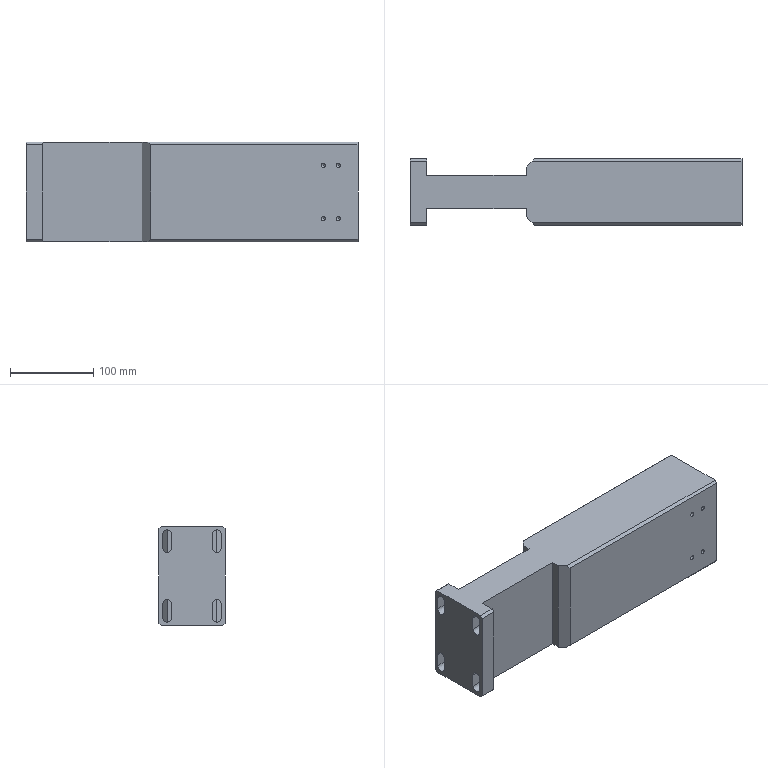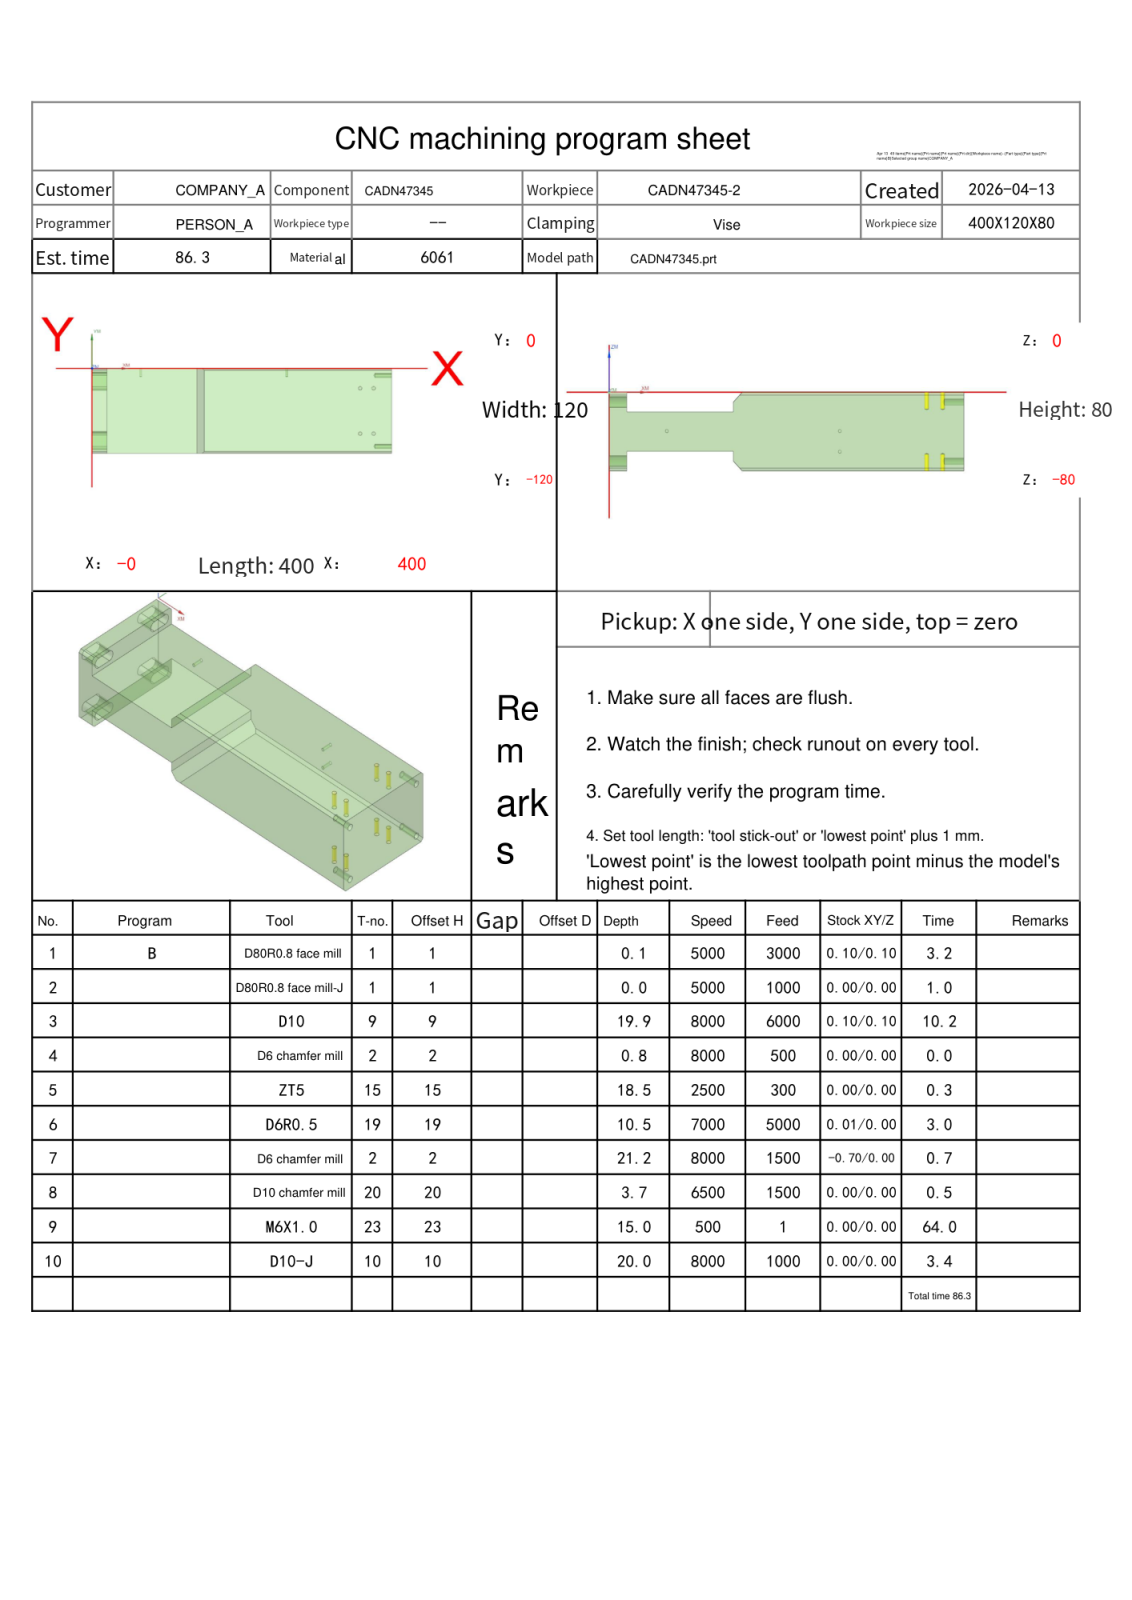NC program | NX | posted by the shop | part box 400 x 80 x 120 mm
Lines 148 to 1360 of 4568:
N3 T09 M06
(D10  D=10. R=0. H=09 ce=0.10 di=0.10)
G00 G90 G54 X91.621 Y-134.5 M03 S8000
G43 H09 Z14.8
M08
Z.404
G01 Z-.796 F6000.
Y-127.08
G03 X84.621 Y-120.08 I-7. J0.0
G01 X26.087
X25.177
G02 X24.48 Y-122.521 I-5.247 J.18
X24.167 Y-123. I-4.55 J2.62
G01 X23.918
G02 X20. Y-124.337 I-3.965 J5.21
G01 X.08
Y-123.
X-.08
Y-122.937
X.08 Y-122.938
X1.48 Y-122.937
X20.
G03 X25.099 Y-117.903 I-.047 J5.147
G01 X25.117 Y-117.802
X25.179 Y-117.08
X25.18 Y-116.774
Y-116.579
Y-116.189
Y-114.405
X25.179 Y-113.513
Y-3.812
X25.178 Y-2.913
X25.116 Y-2.19
X25.099 Y-2.097
G03 X20. Y2.937 I-5.146 J-.113
G01 X1.48
X.08 Y2.938
X-.08 Y2.937
Y3.
X.08
Y4.337
X20.013
G02 X23.918 Y3. I-.06 J-6.547
G01 X24.154
G02 X24.452 Y2.547 I-4.274 J-3.135
X25.176 Y.08 I-4.572 J-2.682
G01 X26.087
X134.898
X135.207
X141.852
G02 X142.877 Y3. I5.492 J-.286
G01 X145.194
G02 X149.133 Y4.337 I3.939 J-5.134
G01 X399.92
Y3.
X400.08
Y2.937
X399.92 Y2.938
X149.133 Y2.937
G03 X144.063 Y-2.133 I0.0 J-5.071
G01 Y-117.867
G03 X149.133 Y-122.937 I5.071 J0.0
G01 X398.52
X399.92
X400.08
Y-123.
X399.92
Y-124.337
X149.133
G02 X145.194 Y-123. I0.0 J6.471
G01 X142.86
G02 X142.513 Y-122.469 I4.246 J3.15
G01 X142.281 Y-122.023
X142.117 Y-121.559
X141.891 Y-120.662
X141.789 Y-120.08
X135.207
X134.898
X87.635
G02 X86.822 Y-119.662 I.001 J1.
G01 X82.419 Y-113.498
G03 X81.607 Y-113.08 I-.813 J-.582
G01 X33.175
G02 X32.179 Y-112.084 I.004 J1.
G01 Y-7.916
G02 X33.175 Y-6.92 I1. J-.004
G01 X134.896
X135.205
X136.067
G02 X137.063 Y-7.916 I-.004 J-1.
G01 Y-112.084
G02 X136.067 Y-113.08 I-1. J.004
G01 X135.205
X134.896
X87.635
G02 X86.822 Y-112.662 I.001 J1.
G01 X82.419 Y-106.498
G03 X81.606 Y-106.08 I-.813 J-.582
G01 X40.174
G02 X39.179 Y-105.085 I.005 J1.
G01 Y-14.915
G02 X40.174 Y-13.92 I1. J-.005
G01 X129.067
G02 X130.063 Y-14.915 I-.005 J-1.
G01 Y-105.085
G02 X129.067 Y-106.08 I-1. J.005
G01 X87.635
G02 X86.822 Y-105.662 I.001 J1.
G01 X82.419 Y-99.498
G03 X81.606 Y-99.08 I-.813 J-.582
G01 X47.174
G02 X46.179 Y-98.085 I.005 J1.
G01 Y-21.915
G02 X47.174 Y-20.92 I1. J-.005
G01 X122.067
G02 X123.063 Y-21.915 I-.005 J-1.
G01 Y-98.085
G02 X122.067 Y-99.08 I-1. J.005
G01 X87.635
G02 X86.822 Y-98.662 I0.0 J1.
G01 X82.419 Y-92.498
G03 X81.606 Y-92.08 I-.813 J-.582
G01 X54.174
G02 X53.179 Y-91.085 I.005 J1.
G01 Y-28.915
G02 X54.174 Y-27.92 I1. J-.005
G01 X115.068
G02 X116.063 Y-28.915 I-.005 J-1.
G01 Y-91.085
G02 X115.068 Y-92.08 I-1. J.005
G01 X87.635
G02 X86.822 Y-91.662 I0.0 J1.
G01 X82.419 Y-85.498
G03 X81.606 Y-85.08 I-.814 J-.582
G01 X61.173
G02 X60.179 Y-84.085 I.005 J1.
G01 Y-35.915
G02 X61.173 Y-34.92 I1. J-.005
G01 X108.068
G02 X109.063 Y-35.915 I-.005 J-1.
G01 Y-84.085
G02 X108.068 Y-85.08 I-1. J.005
G01 X87.635
G02 X86.822 Y-84.662 I0.0 J1.
G01 X82.419 Y-78.498
G03 X81.606 Y-78.08 I-.814 J-.582
G01 X68.173
G02 X67.179 Y-77.085 I.005 J1.
G01 Y-42.915
G02 X68.173 Y-41.92 I1. J-.005
G01 X101.068
G02 X102.063 Y-42.915 I-.005 J-1.
G01 Y-77.085
G02 X101.068 Y-78.08 I-1. J.005
G01 X87.635
G02 X86.822 Y-77.662 I0.0 J1.
G01 X82.42 Y-71.499
G03 X81.606 Y-71.08 I-.814 J-.582
G01 X75.173
G02 X74.179 Y-70.085 I.005 J1.
G01 Y-49.915
G02 X75.173 Y-48.92 I1. J-.005
G01 X94.068
G02 X95.063 Y-49.915 I-.005 J-1.
G01 Y-70.085
G02 X94.068 Y-71.08 I-1. J.005
G01 X87.635
G02 X86.822 Y-70.661 I0.0 J1.
G01 X82.344 Y-64.391
G03 X81.854 Y-64.026 I-.814 J-.581
G02 X81.179 Y-63.085 I.324 J.946
G01 Y-56.915
G02 X82.173 Y-55.92 I1. J-.005
G01 X87.068
G02 X88.063 Y-56.915 I-.005 J-1.
G01 Y-63.085
G02 X87.068 Y-64.08 I-1. J.005
G01 X84.621
X84.121
G03 X77.121 Y-71.08 I0.0 J-7.
G01 Z.404
G00 Z3.
G01 X91.621 Y-134.5
G00 Z-.392
G01 Z-1.592
Y-127.08
G03 X84.621 Y-120.08 I-7. J0.0
G01 X25.177
G02 X19.93 Y-125.151 I-5.247 J.18
G01 X19.92
X0.0
X-.085 Y-125.156
X-.08 Y-125.071
Y-123.733
X0.0
X.003
X.08
X20.
G03 X25.1 Y-118.613 I-.021 J5.121
G01 Y-118.592
Y-117.897
X25.117 Y-117.802
X25.179 Y-117.08
X25.18 Y-116.774
Y-116.579
Y-116.189
Y-115.297
Y-114.405
X25.179 Y-113.513
Y-3.812
X25.178 Y-2.913
X25.116 Y-2.19
X25.1 Y-2.103
Y-1.408
Y-1.387
G03 X20. Y3.733 I-5.121 J0.0
G01 X.08
X.007
X0.0
X-.08
Y5.071
X-.085 Y5.156
X0.0 Y5.151
X19.922
X20.504 Y5.134
X20.828 Y5.08
G02 X25.176 Y.08 I-.948 J-5.215
G01 X33.175
X134.898
X135.27
X141.852
G02 X144.103 Y4.236 I5.492 J-.287
X147.426 Y5.157 I3.324 J-5.531
X147.72 Y5.151 I0.0 J-6.453
G01 X400.
X400.085 Y5.156
X400.08 Y5.071
Y3.733
X400.
X399.994
X399.92
X148.337
G03 X143.267 Y-1.337 I0.0 J-5.071
G01 Y-118.663
G03 X148.337 Y-123.733 I5.071 J0.0
G01 X399.92
X400.08
Y-124.215
Y-125.071
X400.085 Y-125.156
X400. Y-125.151
X147.717
X146.821 Y-125.129
G02 X142.513 Y-122.469 I.285 J5.279
G01 X142.281 Y-122.023
X142.117 Y-121.559
X141.891 Y-120.662
X141.789 Y-120.08
X135.207
X134.898
X87.635
G02 X86.822 Y-119.662 I.001 J1.
G01 X82.419 Y-113.498
G03 X81.607 Y-113.08 I-.813 J-.582
G01 X33.175
G02 X32.179 Y-112.083 I.003 J1.
G01 Y-7.917
G02 X33.175 Y-6.92 I1. J-.003
G01 X134.896
X135.27
G02 X136.267 Y-7.917 I-.003 J-1.
G01 Y-112.083
G02 X135.265 Y-113.082 I-1.002 J.004
G01 X135.205 Y-113.08
X134.896
X87.635
G02 X86.822 Y-112.662 I.001 J1.
G01 X82.419 Y-106.498
G03 X81.606 Y-106.08 I-.813 J-.582
G01 X40.175
G02 X39.179 Y-105.084 I.004 J1.
G01 Y-14.916
G02 X40.175 Y-13.92 I1. J-.004
G01 X128.271
G02 X129.267 Y-14.916 I-.004 J-1.
G01 Y-105.084
G02 X128.271 Y-106.08 I-1. J.004
G01 X87.635
G02 X86.822 Y-105.662 I0.0 J1.
G01 X82.419 Y-99.498
G03 X81.606 Y-99.08 I-.813 J-.582
G01 X47.174
G02 X46.179 Y-98.084 I.004 J1.
G01 Y-21.916
G02 X47.174 Y-20.92 I1. J-.004
G01 X121.271
G02 X122.267 Y-21.916 I-.004 J-1.
G01 Y-98.084
G02 X121.271 Y-99.08 I-1. J.004
G01 X87.635
G02 X86.822 Y-98.662 I0.0 J1.
G01 X82.419 Y-92.498
G03 X81.606 Y-92.08 I-.813 J-.582
G01 X54.174
G02 X53.179 Y-91.085 I.004 J1.
G01 Y-28.915
G02 X54.174 Y-27.92 I1. J-.004
G01 X114.271
G02 X115.267 Y-28.915 I-.004 J-1.
G01 Y-91.085
G02 X114.271 Y-92.08 I-1. J.004
G01 X87.635
G02 X86.822 Y-91.662 I0.0 J1.
G01 X82.419 Y-85.498
G03 X81.606 Y-85.08 I-.814 J-.582
G01 X61.174
G02 X60.179 Y-84.085 I.005 J1.
G01 Y-35.915
G02 X61.174 Y-34.92 I1. J-.005
G01 X107.271
G02 X108.267 Y-35.915 I-.005 J-1.
G01 Y-84.085
G02 X107.271 Y-85.08 I-1. J.005
G01 X87.635
G02 X86.822 Y-84.662 I0.0 J1.
G01 X82.419 Y-78.499
G03 X81.606 Y-78.08 I-.814 J-.582
G01 X68.174
G02 X67.179 Y-77.085 I.005 J1.
G01 Y-42.915
G02 X68.174 Y-41.92 I1. J-.005
G01 X100.271
G02 X101.267 Y-42.915 I-.005 J-1.
G01 Y-77.085
G02 X100.271 Y-78.08 I-1. J.005
G01 X87.635
G02 X86.822 Y-77.662 I0.0 J1.
G01 X82.42 Y-71.499
G03 X81.606 Y-71.08 I-.814 J-.581
G01 X75.174
G02 X74.179 Y-70.085 I.005 J1.
G01 Y-49.915
G02 X75.174 Y-48.92 I1. J-.005
G01 X93.271
G02 X94.267 Y-49.915 I-.005 J-1.
G01 Y-70.085
G02 X93.271 Y-71.08 I-1. J.005
G01 X87.635
G02 X86.822 Y-70.661 I0.0 J1.
G01 X82.344 Y-64.391
G03 X81.854 Y-64.026 I-.814 J-.581
G02 X81.179 Y-63.085 I.324 J.946
G01 Y-56.915
G02 X82.174 Y-55.92 I1. J-.005
G01 X86.272
G02 X87.267 Y-56.915 I-.005 J-1.
G01 Y-63.085
G02 X86.272 Y-64.08 I-1. J.005
G01 X84.621
X84.121
G03 X77.121 Y-71.08 I0.0 J-7.
G01 Z-.392
G00 Z3.
G01 X91.621 Y-134.5
G00 Z-1.188
G01 Z-2.388
Y-127.08
G03 X84.621 Y-120.08 I-7. J0.0
G01 X25.177
G02 X19.93 Y-125.151 I-5.247 J.18
G01 X19.92
X0.0
X-.085 Y-125.156
X-.08 Y-125.071
Y-124.529
X0.0
X.01
X.08
X20.
G03 X25.1 Y-119.388 I-.067 J5.167
G01 Y-117.897
X25.117 Y-117.802
X25.179 Y-117.08
X25.18 Y-116.774
Y-116.579
Y-116.189
Y-114.405
X25.179 Y-113.513
Y-3.812
X25.178 Y-2.913
X25.116 Y-2.19
X25.1 Y-2.103
Y-.612
G03 X20. Y4.529 I-5.167 J-.025
G01 X.08
X.012
X0.0
X-.08
Y5.071
X-.085 Y5.156
X0.0 Y5.151
X19.922
X20.504 Y5.134
X20.828 Y5.08
G02 X25.176 Y.08 I-.948 J-5.215
G01 X33.175
X134.898
X135.207
X141.852
G02 X144.103 Y4.236 I5.492 J-.287
X147.426 Y5.157 I3.324 J-5.531
X147.72 Y5.151 I0.0 J-6.453
G01 X400.
X400.085 Y5.156
X400.08 Y5.071
Y4.529
X400.
X399.988
X399.92
X147.541
G03 X142.471 Y-.541 I0.0 J-5.071
G01 Y-119.459
G03 X147.541 Y-124.529 I5.071 J0.0
G01 X399.742
G03 X399.955 Y-124.534 I.214 J5.141
G01 X400.
X400.08
Y-125.071
X400.085 Y-125.156
X400. Y-125.151
X147.717
X146.821 Y-125.129
G02 X142.513 Y-122.469 I.285 J5.279
G01 X142.281 Y-122.023
X142.117 Y-121.559
X141.891 Y-120.662
X141.789 Y-120.08
X135.207
X134.898
X87.635
G02 X86.822 Y-119.662 I.001 J1.
G01 X82.419 Y-113.498
G03 X81.607 Y-113.08 I-.813 J-.582
G01 X33.175
G02 X32.179 Y-112.084 I.004 J1.
G01 Y-7.916
G02 X33.175 Y-6.92 I1. J-.004
G01 X134.475
G02 X135.471 Y-7.916 I-.004 J-1.
G01 Y-112.084
G02 X134.475 Y-113.08 I-1. J.004
G01 X87.635
G02 X86.822 Y-112.662 I.001 J1.
G01 X82.419 Y-106.498
G03 X81.606 Y-106.08 I-.813 J-.582
G01 X40.174
G02 X39.179 Y-105.085 I.005 J1.
G01 Y-14.915
G02 X40.174 Y-13.92 I1. J-.005
G01 X127.475
G02 X128.471 Y-14.915 I-.005 J-1.
G01 Y-105.085
G02 X127.475 Y-106.08 I-1. J.005
G01 X87.635
G02 X86.822 Y-105.662 I0.0 J1.
G01 X82.419 Y-99.498
G03 X81.606 Y-99.08 I-.813 J-.582
G01 X47.174
G02 X46.179 Y-98.085 I.005 J1.
G01 Y-21.915
G02 X47.174 Y-20.92 I1. J-.005
G01 X120.475
G02 X121.471 Y-21.915 I-.005 J-1.
G01 Y-98.085
G02 X120.475 Y-99.08 I-1. J.005
G01 X87.635
G02 X86.822 Y-98.662 I0.0 J1.
G01 X82.419 Y-92.498
G03 X81.606 Y-92.08 I-.813 J-.582
G01 X54.174
G02 X53.179 Y-91.085 I.005 J1.
G01 Y-28.915
G02 X54.174 Y-27.92 I1. J-.005
G01 X113.475
G02 X114.471 Y-28.915 I-.005 J-1.
G01 Y-91.085
G02 X113.475 Y-92.08 I-1. J.005
G01 X87.635
G02 X86.822 Y-91.662 I0.0 J1.
G01 X82.419 Y-85.498
G03 X81.606 Y-85.08 I-.814 J-.582
G01 X61.174
G02 X60.179 Y-84.085 I.005 J1.
G01 Y-35.915
G02 X61.174 Y-34.92 I1. J-.005
G01 X106.476
G02 X107.471 Y-35.915 I-.005 J-1.
G01 Y-84.085
G02 X106.476 Y-85.08 I-1. J.005
G01 X87.635
G02 X86.822 Y-84.662 I0.0 J1.
G01 X82.419 Y-78.499
G03 X81.606 Y-78.08 I-.814 J-.582
G01 X68.173
G02 X67.179 Y-77.085 I.005 J1.
G01 Y-42.915
G02 X68.173 Y-41.92 I1. J-.005
G01 X99.476
G02 X100.471 Y-42.915 I-.005 J-1.
G01 Y-77.085
G02 X99.476 Y-78.08 I-1. J.005
G01 X87.635
G02 X86.822 Y-77.662 I0.0 J1.
G01 X82.42 Y-71.499
G03 X81.606 Y-71.08 I-.814 J-.582
G01 X75.173
G02 X74.179 Y-70.085 I.005 J1.
G01 Y-49.915
G02 X75.173 Y-48.92 I1. J-.005
G01 X92.476
G02 X93.471 Y-49.915 I-.005 J-1.
G01 Y-70.085
G02 X92.476 Y-71.08 I-1. J.005
G01 X87.635
G02 X86.822 Y-70.661 I0.0 J1.
G01 X82.344 Y-64.391
G03 X81.854 Y-64.026 I-.814 J-.581
G02 X81.179 Y-63.085 I.324 J.946
G01 Y-56.915
G02 X82.173 Y-55.92 I1. J-.005
G01 X85.476
G02 X86.471 Y-56.915 I-.005 J-1.
G01 Y-63.085
G02 X85.476 Y-64.08 I-1. J.005
G01 X84.621
X84.121
G03 X77.121 Y-71.08 I0.0 J-7.
G01 Z-1.188
G00 Z3.
G01 X91.621 Y-134.5
G00 Z-1.984
G01 Z-3.184
Y-127.08
G03 X84.621 Y-120.08 I-7. J0.0
G01 X25.177
X25.1 Y-120.059
Y-119.388
Y-117.897
X25.117 Y-117.802
X25.179 Y-117.08
X25.18 Y-116.774
Y-116.579
Y-116.189
Y-115.297
Y-114.405
X25.179 Y-113.513
Y-3.812
X25.178 Y-2.913
X25.116 Y-2.19
X25.1 Y-2.103
Y-.08
X25.176 Y.08
X32.179
X134.898
X135.207
X141.675
Y0.0
Y-6.92
Y-119.92
Y-120.08
X135.207
X134.898
X87.635
G02 X86.822 Y-119.662 I.001 J1.
G01 X82.419 Y-113.498
G03 X81.607 Y-113.08 I-.813 J-.582
G01 X33.174
G02 X32.179 Y-112.084 I.004 J1.
G01 Y-7.916
G02 X33.174 Y-6.92 I1. J-.004
G01 X133.679
G02 X134.675 Y-7.916 I-.004 J-1.
G01 Y-112.084
G02 X133.679 Y-113.08 I-1. J.004
G01 X87.635
G02 X86.822 Y-112.662 I.001 J1.
G01 X82.419 Y-106.498
G03 X81.606 Y-106.08 I-.813 J-.582
G01 X40.174
G02 X39.179 Y-105.085 I.005 J1.
G01 Y-14.915
G02 X40.174 Y-13.92 I1. J-.005
G01 X126.679
G02 X127.675 Y-14.915 I-.005 J-1.
G01 Y-105.085
G02 X126.679 Y-106.08 I-1. J.005
G01 X87.635
G02 X86.822 Y-105.662 I0.0 J1.
G01 X82.419 Y-99.498
G03 X81.606 Y-99.08 I-.813 J-.582
G01 X47.174
G02 X46.179 Y-98.085 I.005 J1.
G01 Y-21.915
G02 X47.174 Y-20.92 I1. J-.005
G01 X119.679
G02 X120.675 Y-21.915 I-.005 J-1.
G01 Y-98.085
G02 X119.679 Y-99.08 I-1. J.005
G01 X87.635
G02 X86.822 Y-98.662 I0.0 J1.
G01 X82.419 Y-92.498
G03 X81.606 Y-92.08 I-.813 J-.582
G01 X54.174
G02 X53.179 Y-91.085 I.005 J1.
G01 Y-28.915
G02 X54.174 Y-27.92 I1. J-.005
G01 X112.68
G02 X113.675 Y-28.915 I-.005 J-1.
G01 Y-91.085
G02 X112.68 Y-92.08 I-1. J.005
G01 X87.635
G02 X86.822 Y-91.662 I0.0 J1.
G01 X82.419 Y-85.498
G03 X81.606 Y-85.08 I-.814 J-.582
G01 X61.173
G02 X60.179 Y-84.085 I.005 J1.
G01 Y-35.915
G02 X61.173 Y-34.92 I1. J-.005
G01 X105.68
G02 X106.675 Y-35.915 I-.005 J-1.
G01 Y-84.085
G02 X105.68 Y-85.08 I-1. J.005
G01 X87.635
G02 X86.822 Y-84.662 I0.0 J1.
G01 X82.419 Y-78.498
G03 X81.606 Y-78.08 I-.814 J-.582
G01 X68.173
G02 X67.179 Y-77.085 I.005 J1.
G01 Y-42.915
G02 X68.173 Y-41.92 I1. J-.005
G01 X98.68
G02 X99.675 Y-42.915 I-.005 J-1.
G01 Y-77.085
G02 X98.68 Y-78.08 I-1. J.005
G01 X87.635
G02 X86.822 Y-77.662 I0.0 J1.
G01 X82.42 Y-71.499
G03 X81.606 Y-71.08 I-.814 J-.582
G01 X75.173
G02 X74.179 Y-70.085 I.005 J1.
G01 Y-49.915
G02 X75.173 Y-48.92 I1. J-.005
G01 X91.68
G02 X92.675 Y-49.915 I-.005 J-1.
G01 Y-70.085
G02 X91.68 Y-71.08 I-1. J.005
G01 X87.635
G02 X86.822 Y-70.661 I0.0 J1.
G01 X82.344 Y-64.391
G03 X81.854 Y-64.026 I-.814 J-.581
G02 X81.179 Y-63.085 I.324 J.946
G01 Y-56.915
G02 X82.173 Y-55.92 I1. J-.005
G01 X84.68
G02 X85.675 Y-56.915 I-.005 J-1.
G01 Y-63.085
G02 X84.673 Y-64.081 I-1.001 J.005
G01 X84.621 Y-64.08
X84.121
G03 X77.121 Y-71.08 I0.0 J-7.
G01 Z-1.984
G00 Z3.
G01 X91.621 Y-134.5
G00 Z-2.78
G01 Z-3.98
Y-127.08
G03 X84.621 Y-120.08 I-7. J0.0
G01 X25.177
X25.1 Y-120.058
Y-117.897
X25.117 Y-117.802
X25.179 Y-117.08
X25.18 Y-116.774
Y-116.579
Y-116.189
Y-114.405
X25.179 Y-113.513
Y-3.812
X25.178 Y-2.913
X25.116 Y-2.19
X25.1 Y-2.103
Y-.08
X25.176 Y.08
X32.179
X134.898
X135.207
X140.879
Y0.0
Y-6.92
Y-119.92
Y-120.08
X135.207
X134.898
X87.635
G02 X86.822 Y-119.662 I.001 J1.
G01 X82.419 Y-113.498
G03 X81.607 Y-113.08 I-.813 J-.582
G01 X33.174
G02 X32.179 Y-112.085 I.005 J1.
G01 Y-7.915
G02 X33.174 Y-6.92 I1. J-.005
G01 X132.883
G02 X133.879 Y-7.915 I-.005 J-1.
G01 Y-112.085
G02 X132.883 Y-113.08 I-1. J.005
G01 X87.635
G02 X86.822 Y-112.662 I.001 J1.
G01 X82.419 Y-106.498
G03 X81.606 Y-106.08 I-.813 J-.582
G01 X40.174
G02 X39.179 Y-105.085 I.005 J1.
G01 Y-14.915
G02 X40.174 Y-13.92 I1. J-.005
G01 X125.884
G02 X126.879 Y-14.915 I-.005 J-1.
G01 Y-105.085
G02 X125.884 Y-106.08 I-1. J.005
G01 X87.635
G02 X86.822 Y-105.662 I.001 J1.
G01 X82.419 Y-99.498
G03 X81.606 Y-99.08 I-.813 J-.582
G01 X47.173
G02 X46.179 Y-98.085 I.005 J1.
G01 Y-21.915
G02 X47.173 Y-20.92 I1. J-.005
G01 X118.884
G02 X119.879 Y-21.915 I-.005 J-1.
G01 Y-98.085
G02 X118.884 Y-99.08 I-1. J.005
G01 X87.635
G02 X86.822 Y-98.662 I0.0 J1.
G01 X82.419 Y-92.498
G03 X81.606 Y-92.08 I-.813 J-.582
G01 X54.173
G02 X53.179 Y-91.085 I.005 J1.
G01 Y-28.915
G02 X54.173 Y-27.92 I1. J-.005
G01 X111.884
G02 X112.879 Y-28.915 I-.005 J-1.
G01 Y-91.085
G02 X111.884 Y-92.08 I-1. J.005
G01 X87.635
G02 X86.822 Y-91.662 I0.0 J1.
G01 X82.419 Y-85.498
G03 X81.606 Y-85.08 I-.814 J-.582
G01 X61.173
G02 X60.179 Y-84.086 I.006 J1.
G01 Y-35.914
G02 X61.173 Y-34.92 I1. J-.006
G01 X104.884
G02 X105.879 Y-35.914 I-.006 J-1.
G01 Y-84.086
G02 X104.884 Y-85.08 I-1. J.006
G01 X87.635
G02 X86.822 Y-84.662 I0.0 J1.
G01 X82.419 Y-78.499
G03 X81.606 Y-78.08 I-.814 J-.582
G01 X68.173
G02 X67.179 Y-77.086 I.006 J1.
G01 Y-42.914
G02 X68.173 Y-41.92 I1. J-.006
G01 X97.884
G02 X98.879 Y-42.914 I-.006 J-1.
G01 Y-77.086
G02 X97.884 Y-78.08 I-1. J.006
G01 X87.635
G02 X86.822 Y-77.662 I0.0 J1.
G01 X82.42 Y-71.499
G03 X81.606 Y-71.08 I-.814 J-.582
G01 X75.173
G02 X74.179 Y-70.086 I.006 J1.
G01 Y-49.914
G02 X75.173 Y-48.92 I1. J-.006
G01 X90.884
G02 X91.879 Y-49.914 I-.006 J-1.
G01 Y-70.086
G02 X90.884 Y-71.08 I-1. J.006
G01 X87.611
G02 X86.821 Y-70.692 I0.0 J1.
G01 X81.581 Y-63.907
X81.484 Y-63.8
G02 X81.179 Y-63.086 I.694 J.72
G01 Y-56.914
G02 X82.173 Y-55.92 I1. J-.006
G01 X83.884
G02 X84.879 Y-56.914 I-.006 J-1.
G01 Y-63.086
G02 X83.971 Y-64.076 I-1. J.006
G01 X83.471 Y-64.08
G03 X76.471 Y-71.08 I0.0 J-7.
G01 Z-2.78
G00 Z3.
G01 X91.621 Y-134.5
G00 Z-3.576
G01 Z-4.776
Y-127.08
G03 X84.621 Y-120.08 I-7. J0.0
G01 X25.177
X25.1 Y-120.057
Y-117.897
X25.117 Y-117.802
X25.179 Y-117.08
X25.18 Y-116.774
Y-116.579
Y-116.189
Y-115.297
Y-114.405
X25.179 Y-113.513
Y-3.812
X25.178 Y-2.913
X25.116 Y-2.19
X25.1 Y-2.103
Y-.08
X25.176 Y.08
X32.179
X134.898
X135.207
X140.083
Y0.0
Y-6.92
Y-119.92
Y-120.08
X135.207
X134.898
X87.635
G02 X86.822 Y-119.662 I.001 J1.
G01 X82.419 Y-113.498
G03 X81.607 Y-113.08 I-.813 J-.582
G01 X33.173
G02 X32.179 Y-112.085 I.005 J1.
G01 Y-7.915
G02 X33.173 Y-6.92 I1. J-.005
G01 X132.088
G02 X133.083 Y-7.915 I-.005 J-1.
G01 Y-112.085
G02 X132.088 Y-113.08 I-1. J.005
G01 X87.635
G02 X86.822 Y-112.662 I.001 J1.
G01 X82.419 Y-106.498
G03 X81.606 Y-106.08 I-.813 J-.582
G01 X40.173
G02 X39.179 Y-105.085 I.005 J1.
G01 Y-14.915
G02 X40.173 Y-13.92 I1. J-.005
G01 X125.088
G02 X126.083 Y-14.915 I-.005 J-1.
G01 Y-105.085
G02 X125.088 Y-106.08 I-1. J.005
G01 X87.635
G02 X86.822 Y-105.662 I0.0 J1.
G01 X82.419 Y-99.498
G03 X81.606 Y-99.08 I-.813 J-.582
G01 X47.173
G02 X46.179 Y-98.086 I.006 J1.
G01 Y-21.914
G02 X47.173 Y-20.92 I1. J-.006
G01 X118.088
G02 X119.083 Y-21.914 I-.006 J-1.
G01 Y-98.086
G02 X118.088 Y-99.08 I-1. J.006
G01 X87.635
G02 X86.822 Y-98.662 I0.0 J1.
G01 X82.419 Y-92.498
G03 X81.606 Y-92.08 I-.813 J-.582
G01 X54.173
G02 X53.179 Y-91.086 I.006 J1.
G01 Y-28.914
G02 X54.173 Y-27.92 I1. J-.006
G01 X111.088
G02 X112.083 Y-28.914 I-.006 J-1.
G01 Y-91.086
G02 X111.088 Y-92.08 I-1. J.006
G01 X87.635
G02 X86.822 Y-91.662 I0.0 J1.
G01 X82.419 Y-85.498
G03 X81.606 Y-85.08 I-.813 J-.582
G01 X61.173
G02 X60.179 Y-84.086 I.006 J1.
G01 Y-35.914
G02 X61.173 Y-34.92 I1. J-.006
G01 X104.088
G02 X105.083 Y-35.914 I-.006 J-1.
G01 Y-84.086
G02 X104.088 Y-85.08 I-1. J.006
G01 X87.635
G02 X86.822 Y-84.662 I0.0 J1.
G01 X82.419 Y-78.499
G03 X81.606 Y-78.08 I-.814 J-.582
G01 X68.173
G02 X67.179 Y-77.086 I.006 J1.
G01 Y-42.914
G02 X68.173 Y-41.92 I1. J-.006
G01 X97.089
G02 X98.083 Y-42.914 I-.006 J-1.
G01 Y-77.086
G02 X97.089 Y-78.08 I-1. J.006
G01 X87.635
G02 X86.822 Y-77.662 I0.0 J1.
G01 X82.42 Y-71.499
G03 X81.606 Y-71.08 I-.814 J-.582
G01 X75.173
G02 X74.179 Y-70.086 I.006 J1.
G01 Y-49.914
G02 X75.173 Y-48.92 I1. J-.006
G01 X90.089
G02 X91.083 Y-49.914 I-.006 J-1.
G01 Y-70.086
G02 X90.089 Y-71.08 I-1. J.006
G01 X87.638
G02 X86.822 Y-70.658 I0.0 J1.
G01 X82.409 Y-64.415
G03 X81.886 Y-64.036 I-.816 J-.577
G02 X81.179 Y-63.086 I.293 J.956
G01 Y-56.914
G02 X82.172 Y-55.92 I1. J-.006
G01 X83.089
G02 X84.083 Y-56.914 I-.006 J-1.
G01 Y-63.086
G02 X83.271 Y-64.062 I-1. J.006
G01 X83.089 Y-64.08
X82.773
G03 X75.773 Y-71.08 I0.0 J-7.
G01 Z-3.576
G00 Z3.
G01 X91.621 Y-134.5
G00 Z-4.372
G01 Z-5.572
Y-127.08
G03 X84.621 Y-120.08 I-7. J0.0
G01 X25.177
X25.1 Y-120.056
Y-117.897
X25.117 Y-117.802
X25.179 Y-117.08
X25.18 Y-116.774
Y-116.579
Y-116.189
Y-115.297
Y-114.405
X25.179 Y-113.513
Y-3.812
X25.178 Y-2.913
X25.116 Y-2.19
X25.1 Y-2.103
Y-.08
X25.176 Y.08
X32.179
X134.898
X135.207
X139.287
Y0.0
Y-6.92
Y-119.92
Y-120.08
X135.207
X134.898
X87.635
G02 X86.822 Y-119.662 I.001 J1.
G01 X82.419 Y-113.498
G03 X81.607 Y-113.08 I-.813 J-.582
G01 X33.173
G02 X32.179 Y-112.086 I.006 J1.
G01 Y-7.914
G02 X33.173 Y-6.92 I1. J-.006
G01 X131.292
G02 X132.287 Y-7.914 I-.006 J-1.
G01 Y-112.086
G02 X131.292 Y-113.08 I-1. J.006
G01 X87.635
G02 X86.822 Y-112.662 I.001 J1.
G01 X82.419 Y-106.498
G03 X81.606 Y-106.08 I-.813 J-.582
G01 X40.173
G02 X39.179 Y-105.086 I.006 J1.
G01 Y-14.914
G02 X40.173 Y-13.92 I1. J-.006
G01 X124.292
G02 X125.287 Y-14.914 I-.006 J-1.
G01 Y-105.086
G02 X124.292 Y-106.08 I-1. J.006
G01 X87.635
G02 X86.822 Y-105.662 I0.0 J1.
G01 X82.419 Y-99.498
G03 X81.606 Y-99.08 I-.813 J-.582
G01 X47.173
G02 X46.179 Y-98.086 I.006 J1.
G01 Y-21.914
G02 X47.173 Y-20.92 I1. J-.006
G01 X117.293
G02 X118.287 Y-21.914 I-.006 J-1.
G01 Y-98.086
G02 X117.293 Y-99.08 I-1. J.006
G01 X87.635
G02 X86.822 Y-98.662 I0.0 J1.
G01 X82.419 Y-92.498
G03 X81.606 Y-92.08 I-.813 J-.582
G01 X54.173
G02 X53.179 Y-91.086 I.006 J1.
G01 Y-28.914
G02 X54.173 Y-27.92 I1. J-.006
G01 X110.293
G02 X111.287 Y-28.914 I-.006 J-1.
G01 Y-91.086
G02 X110.293 Y-92.08 I-1. J.006
G01 X87.635
G02 X86.822 Y-91.662 I0.0 J1.
G01 X82.419 Y-85.498
G03 X81.606 Y-85.08 I-.814 J-.582
G01 X61.172
G02 X60.179 Y-84.086 I.006 J1.
G01 Y-35.914
G02 X61.172 Y-34.92 I1. J-.006
G01 X103.293
G02 X104.287 Y-35.914 I-.006 J-1.
G01 Y-84.086
G02 X103.293 Y-85.08 I-1. J.006
G01 X87.635
G02 X86.822 Y-84.662 I0.0 J1.
G01 X82.419 Y-78.498
G03 X81.606 Y-78.08 I-.814 J-.582
G01 X68.172
G02 X67.179 Y-77.086 I.006 J1.
G01 Y-42.914
G02 X68.172 Y-41.92 I1. J-.006
G01 X96.293
G02 X97.287 Y-42.914 I-.006 J-1.
G01 Y-77.086
G02 X96.293 Y-78.08 I-1. J.006
G01 X87.635
G02 X86.822 Y-77.662 I0.0 J1.
G01 X82.42 Y-71.499
G03 X81.606 Y-71.08 I-.814 J-.582
G01 X75.172
G02 X74.179 Y-70.086 I.006 J1.
G01 Y-49.914
G02 X75.172 Y-48.92 I1. J-.006
G01 X89.293
G02 X90.287 Y-49.914 I-.006 J-1.
G01 Y-70.086
G02 X89.293 Y-71.08 I-1. J.006
G01 X87.638
G02 X86.822 Y-70.658 I0.0 J1.
G01 X82.409 Y-64.415
G03 X81.886 Y-64.036 I-.816 J-.578
G02 X81.179 Y-63.086 I.293 J.956
G01 Y-56.914
G02 X82.172 Y-55.92 I1. J-.006
G01 X82.293
G02 X83.287 Y-56.914 I-.006 J-1.
G01 Y-63.086
G02 X82.567 Y-64.04 I-1. J.006
X82.293 Y-64.08 I-.28 J.96
G01 X82.071 Y-64.074
G03 X81.315 Y-64.033 I-.755 J-6.959
X74.356 Y-70.278 I0.0 J-7.
G01 Z-4.372
G00 Z3.
G01 X91.621 Y-134.5
G00 Z-5.168
G01 Z-6.368
Y-127.08
G03 X84.621 Y-120.08 I-7. J0.0
G01 X25.177
X25.1 Y-120.055
Y-117.897
X25.117 Y-117.802
X25.179 Y-117.08
X25.18 Y-116.774
Y-116.579
Y-116.189
Y-115.297
Y-114.405
X25.179 Y-113.513
Y-3.812
X25.178 Y-2.913
X25.116 Y-2.19
X25.1 Y-2.103
Y-.08
X25.176 Y.08
X32.179
X134.898
X135.207
X138.491
Y-.003
Y-119.92
Y-120.08
X135.207
X134.898
X87.635
G02 X86.822 Y-119.662 I.001 J1.
G01 X82.419 Y-113.498
G03 X81.607 Y-113.08 I-.813 J-.582
G01 X33.173
G02 X32.179 Y-112.086 I.006 J1.
G01 Y-7.914
G02 X33.173 Y-6.92 I1. J-.006
G01 X130.497
G02 X131.491 Y-7.914 I-.006 J-1.
G01 Y-112.086
G02 X130.497 Y-113.08 I-1. J.006
G01 X87.635
G02 X86.822 Y-112.662 I.001 J1.
G01 X82.419 Y-106.498
G03 X81.606 Y-106.08 I-.813 J-.582
G01 X40.172
G02 X39.179 Y-105.086 I.006 J1.
G01 Y-14.914
G02 X40.172 Y-13.92 I1. J-.006
G01 X123.497
G02 X124.491 Y-14.914 I-.006 J-1.
G01 Y-105.086
G02 X123.497 Y-106.08 I-1. J.006
G01 X87.635
G02 X86.822 Y-105.662 I.001 J1.
G01 X82.419 Y-99.498
G03 X81.606 Y-99.08 I-.813 J-.582
G01 X47.172
G02 X46.179 Y-98.086 I.006 J1.
G01 Y-21.914
G02 X47.172 Y-20.92 I1. J-.006
G01 X116.497
G02 X117.491 Y-21.914 I-.006 J-1.
G01 Y-98.086
G02 X116.497 Y-99.08 I-1. J.006
G01 X87.635
G02 X86.822 Y-98.662 I0.0 J1.
G01 X82.419 Y-92.498
G03 X81.606 Y-92.08 I-.813 J-.582
G01 X54.172
G02 X53.179 Y-91.086 I.006 J1.
G01 Y-28.914
G02 X54.172 Y-27.92 I1. J-.006
G01 X109.497
G02 X110.491 Y-28.914 I-.006 J-1.
G01 Y-91.086
G02 X109.497 Y-92.08 I-1. J.006
G01 X87.635
G02 X86.822 Y-91.662 I0.0 J1.
G01 X82.419 Y-85.498
G03 X81.606 Y-85.08 I-.814 J-.582
G01 X61.172
G02 X60.179 Y-84.087 I.006 J1.
G01 Y-35.913
G02 X61.172 Y-34.92 I1. J-.006
G01 X102.497
G02 X103.491 Y-35.913 I-.006 J-1.
G01 Y-84.087
G02 X102.497 Y-85.08 I-1. J.006
G01 X87.635
G02 X86.822 Y-84.662 I0.0 J1.
G01 X82.419 Y-78.498
G03 X81.606 Y-78.08 I-.814 J-.582
G01 X68.172
G02 X67.179 Y-77.087 I.007 J1.
G01 Y-42.913
G02 X68.172 Y-41.92 I1. J-.007
G01 X95.497
G02 X96.491 Y-42.913 I-.007 J-1.
G01 Y-77.087
G02 X95.497 Y-78.08 I-1. J.007
G01 X87.635
G02 X86.822 Y-77.662 I0.0 J1.
G01 X82.42 Y-71.499
G03 X81.606 Y-71.08 I-.814 J-.582
G01 X75.172
G02 X74.179 Y-70.087 I.007 J1.
G01 Y-49.913
G02 X75.172 Y-48.92 I1. J-.007
G01 X88.497
G02 X89.491 Y-49.913 I-.007 J-1.
G01 Y-70.087
G02 X88.497 Y-71.08 I-1. J.007
G01 X87.615
G02 X86.821 Y-70.687 I0.0 J1.
G01 X81.989 Y-64.362
G03 X81.56 Y-64.039 I-.794 J-.607
G02 X81.179 Y-63.485 I.219 J.559
G01 Y-56.515
G02 X81.773 Y-55.92 I.6 J-.005
G01 X81.896
G02 X82.491 Y-56.515 I-.005 J-.6
G01 Y-63.485
G02 X82.093 Y-64.045 I-.6 J.005
X81.896 Y-64.08 I-.203 J.565
G01 X81.773
X81.6 Y-64.053
G03 X79.52 Y-63.737 I-2.08 J-6.684
X72.836 Y-68.656 I0.0 J-7.
G01 Z-5.168
G00 Z3.
G01 X91.621 Y-134.5
G00 Z-5.964
G01 Z-7.164
Y-127.08
G03 X84.621 Y-120.08 I-7. J0.0
G01 X25.177
X25.1 Y-120.054
Y-117.897
X25.117 Y-117.802
X25.179 Y-117.08
X25.18 Y-116.774
Y-116.579
Y-116.189